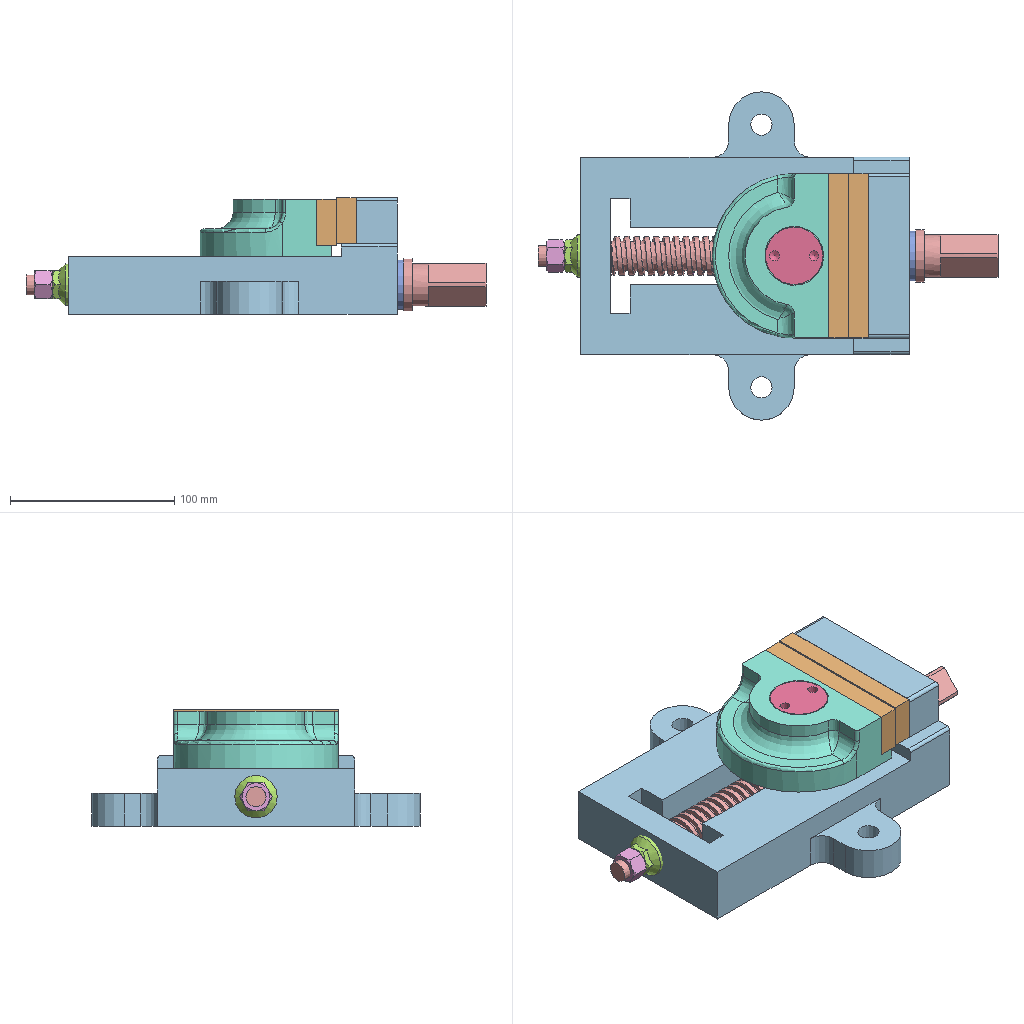Assembly | NX | 13 different items | 17 placed | box 280 x 200 x 71 mm
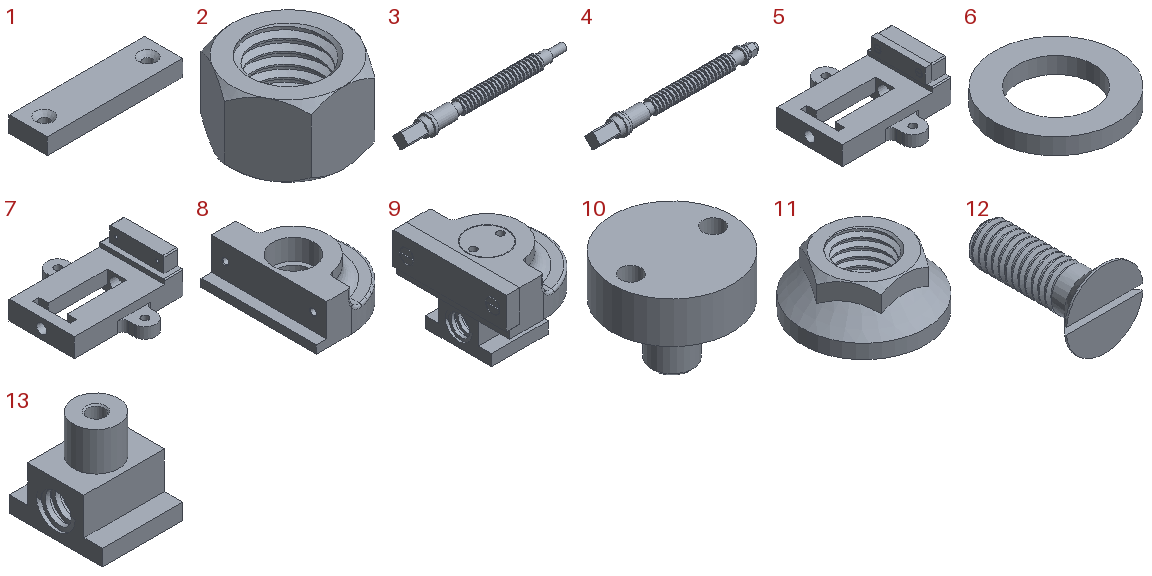Parts list (item | quantity | parent item | size | volume | features):
1 | x2 | in 5, 9 | 100 x 28 x 12 mm | 32422 mm3 | features DATUM_CSYS 2, CHAMFER 1, EXTRUDE 1, SKETCH 1
2 | x1 | in 4 | 19.63 x 17 x 11 mm | 1644 mm3 | features DATUM_CSYS 3, EXTRACT_DATUM_AXIS 2, EXTRACT_STRING 2, SKETCH 2, SWP104 2, EXTRUDE 1, HOLE PACKAGE 1, Instance Feature 1, Mirror Feature 1, SIMPLE HOLE 1, SYMBOLIC_THREAD 1, THREADS 1
3 | x1 | in 4 | 280 x 32 x 32 mm | 99870 mm3 | features CYLINDER 6, DATUM_CSYS 2, RECT_GROOVE 2, SKETCH 2, DATUM_ON_PATH 1, EXTRUDE 1, HELIX 1, SKIN 1, SUBTRACT 1, SYMBOLIC_THREAD 1
4 | x1 | - | 280 x 32 x 32 mm | 105505 mm3 | features DATUM_CSYS 9, CYLINDER 8, SKETCH 6, EXTRUDE 4, SYMBOLIC_THREAD 3, EXTRACT_DATUM_AXIS 2, EXTRACT_STRING 2, HOLE PACKAGE 2, RECT_GROOVE 2, SIMPLE HOLE 2, SWP104 2, THREADS 2, CHAMFER 1, CONE 1, DATUM_ON_PATH 1, DELETE FACE 1, HELIX 1, INTERSECT 1, Instance Feature 1, Mirror Feature 1, SKIN 1, SUBTRACT 1
5 | x1 | - | 200 x 200 x 71 mm | 790053 mm3 | features DATUM_CSYS 13, SKETCH 10, EXTRUDE 9, SIMPLE HOLE 4, BLEND 3, HOLE PACKAGE 3, CHAMFER 2, EXTRACT_DATUM_AXIS 2, EXTRACT_DATUM_PLANE 2, EXTRACT_FACE 2, EXTRACT_STRING 2, SYMBOLIC_THREAD 2, BLOCK 1, CYLINDER 1, Instance Feature 1, Mirror Feature 1, SWP104 1, THREADS 1
6 | x1 | in 4 | 30 x 30 x 4 mm | 1752 mm3 | features DATUM_CSYS 2, EXTRUDE 1, SKETCH 1
7 | x1 | in 5 | 200 x 200 x 71 mm | 757054 mm3 | features DATUM_CSYS 8, EXTRUDE 7, SKETCH 7, SIMPLE HOLE 4, BLEND 3, HOLE PACKAGE 3, EXTRACT_DATUM_AXIS 2, EXTRACT_DATUM_PLANE 2, EXTRACT_FACE 2, EXTRACT_STRING 2, SYMBOLIC_THREAD 2, BLOCK 1, Instance Feature 1, Mirror Feature 1
8 | x1 | in 9 | 80 x 100 x 35 mm | 145409 mm3 | features BLEND 3, DATUM_CSYS 2, EXTRUDE 2, HOLE PACKAGE 2, SIMPLE HOLE 2, SYMBOLIC_THREAD 2, BLOCK 1, CBORE_HOLE 1, DELETE FACE 1, SKETCH 1, SWP104 1
9 | x1 | - | 83 x 100 x 69 mm | 255059 mm3 | features DATUM_CSYS 13, SKETCH 9, EXTRUDE 6, SIMPLE HOLE 6, HOLE PACKAGE 5, SYMBOLIC_THREAD 4, BLEND 3, CHAMFER 3, SWP104 3, BLOCK 2, CBORE_HOLE 1, CYLINDER 1, DATUM_ON_PATH 1, DELETE FACE 1, HELIX 1, SKIN 1, SUBTRACT 1, THREADS 1
10 | x1 | in 9 | 35 x 35 x 28 mm | 12801 mm3 | features DATUM_CSYS 3, SIMPLE HOLE 2, SKETCH 2, CHAMFER 1, HOLE PACKAGE 1, SWP104 1, SYMBOLIC_THREAD 1
11 | x1 | in 4 | 26 x 26 x 11 mm | 3067 mm3 | features CYLINDER 2, DATUM_CSYS 2, CHAMFER 1, CONE 1, DELETE FACE 1, EXTRUDE 1, HOLE PACKAGE 1, INTERSECT 1, SIMPLE HOLE 1, SKETCH 1, SYMBOLIC_THREAD 1, THREADS 1
12 | x4 | in 5, 9 | 11.557 x 18 x 11.6 mm | 532.719 mm3 | features DATUM_CSYS 3, SKETCH 2, CHAMFER 1, CYLINDER 1, EXTRUDE 1, SWP104 1, THREADS 1
13 | x1 | in 9 | 50.001 x 58 x 57 mm | 63589 mm3 | features DATUM_CSYS 3, SKETCH 3, EXTRUDE 2, HOLE PACKAGE 2, SIMPLE HOLE 2, BLOCK 1, DATUM_ON_PATH 1, HELIX 1, SKIN 1, SUBTRACT 1, SYMBOLIC_THREAD 1
Mates (type | each side: item.copy, entity, surface, feature):
In the top assembly
Fix | 5.1 component
Touch | 8.1 face plane Block(1) | 7.1 face plane Block(1)
Center22 | 1.1 face plane Extrude(2) | 1.1 face plane Extrude(2) | 1.1 face plane Extrude(2) | 1.1 face plane Extrude(2)
Distance | 1.1 face plane Extrude(2) | 1.1 face plane Extrude(2)
Touch | 3.1 face cylinder Cylinder(4) | 7.1 face cylinder Ø25 Hole(13)
Touch | 6.1 face plane Extrude(1) | 7.1 face plane Block(1)
Parallel | 4.1 plane | assembly plane
In subassembly 4
Fix | 3.1 component
Touch | 6.1 face cylinder Extrude(1) | 3.1 face cylinder Cylinder(5)
Touch | 6.1 face plane Extrude(1) | 3.1 face plane Cylinder(6)
Parallel | 6.1 | 4.2 plane
Touch | 11.1 face cylinder M12 x 1.75 Threaded Hole(9) | 3.1 face cylinder Cylinder(2)
Touch | 11.1 face plane Extrude(2) | 3.1 face plane Cylinder(3)
Parallel | 11.1 | 4.2 plane
Touch | 2.1 face cylinder M12 x 1.75 Threaded Hole(6) | 3.1 face cylinder Cylinder(2)
Touch | 2.1 face plane Extrude(1) | 11.1 face plane Extrude(2)
Parallel | 2.1 | 4.2 plane
In subassembly 5
Fix | 7.1 component
Touch | 1.1 face plane Extrude(2) | 7.1 face plane Extrude(4)
Touch | 1.1 face cylinder Extrude(2) | 7.1 face cylinder M6 x 1.0 Threaded Hole(14) | 2 times
Touch | 12.1 face plane Cylinder(1) | 1.1 face plane Extrude(2) | 2 times
Touch | 12.1 face cylinder Cylinder(1) | 1.1 face cylinder Extrude(2) | 2 times
Parallel | 12.1 face plane Extrude(3) | 1.1 face plane Extrude(2) | 2 times
In subassembly 9
Fix | 8.1 component
Touch | 1.1 face plane Extrude(2) | 8.1 face plane Extrude(4)
Touch | 1.1 face cylinder Extrude(2) | 8.1 face cylinder M6 x 1.0 Threaded Hole(10) | 2 times
Touch | 12.1 face cylinder Cylinder(1) | 1.1 face cylinder Extrude(2) | 2 times
Touch | 12.1 face plane Cylinder(1) | 1.1 face plane Extrude(2) | 2 times
Parallel | 12.1 face plane Extrude(3) | 1.1 face plane Extrude(2) | 2 times
Touch | 13.1 face cylinder Extrude(3) | 8.1 face surfaceofrevolution Edge Blend(8)
Distance | 13.1 face plane Block(1) | 8.1 face plane Block(1)
Parallel | 13.1 face plane Block(1) | 8.1 face plane Block(1)
Touch | 10.1 face cylinder Revolve(1) | 8.1 face cylinder Ø28 Counterbored Hole(6)
Touch | 10.1 face plane Revolve(1) | 13.1 face plane Extrude(3)
Parallel | 10.1 | 8.1 face plane Block(1)